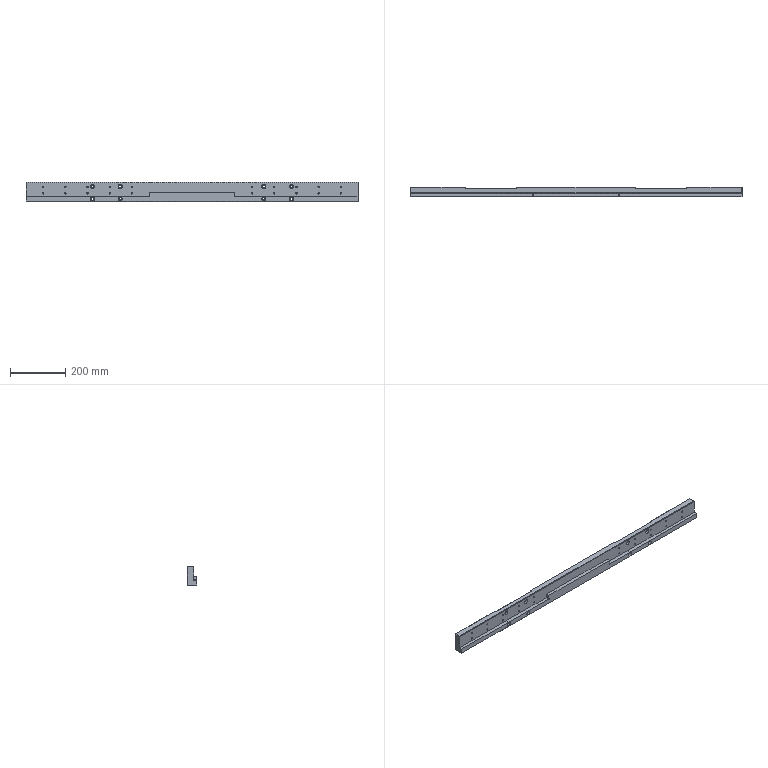Part | STEP file | traverse rod | 1 solid | 198 faces | box 1200 x 35 x 70 mm | volume 2126104 mm3 | cylinder 92 | cone 56 | plane 50 | commonest cylinder face diameters 5 x52 9 x16 15 x16 6.8 x8